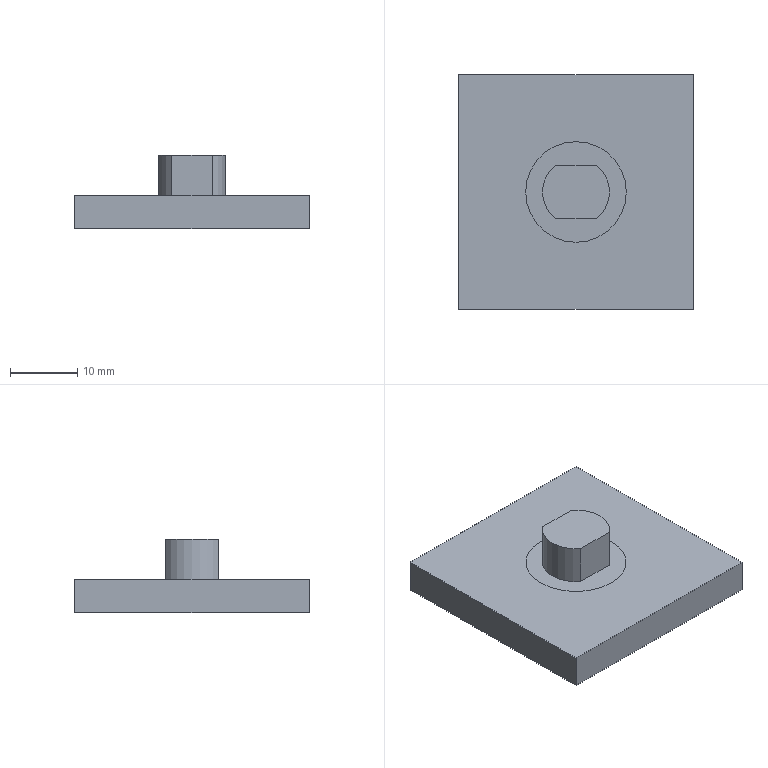NC program | NX | posted with a generic post | part box 35 x 35 x 11 mm
Whole program:
N10 G17 G21 G94 G90
(HOLE_MILLING , TOOL : D10)
N12 T10 M6
N14 G54
N16 G17 G0 G90 X0. Y0. S7000 M3
N18 G43 Z30. H10
N20 Z0.5
N22 G94 G3 X1.25 Y-1.25 R1.25 F2000.
N24 X2.5 Y0. R1.25
N26 X2.5 Y0. Z-0.5 I-2.5 J0.
N28 X2.5 Y0. Z-1.5 I-2.5 J0.
N30 X2.5 Y0. Z-2.5 I-2.5 J0.
N32 X2.5 Y0. Z-3.5 I-2.5 J0.
N34 X2.5 Y0. Z-4.5 I-2.5 J0.
N36 X-2.5 Y0. Z-5. I-2.5 J0.
N38 X0. Y-2.5 R2.5
N40 X-2.5 Y0. R-2.5
N42 X-1.25 Y-1.25 R1.25
N44 X0. Y0. R1.25
N46 G0 Z30.
N48 M5
N50 M2